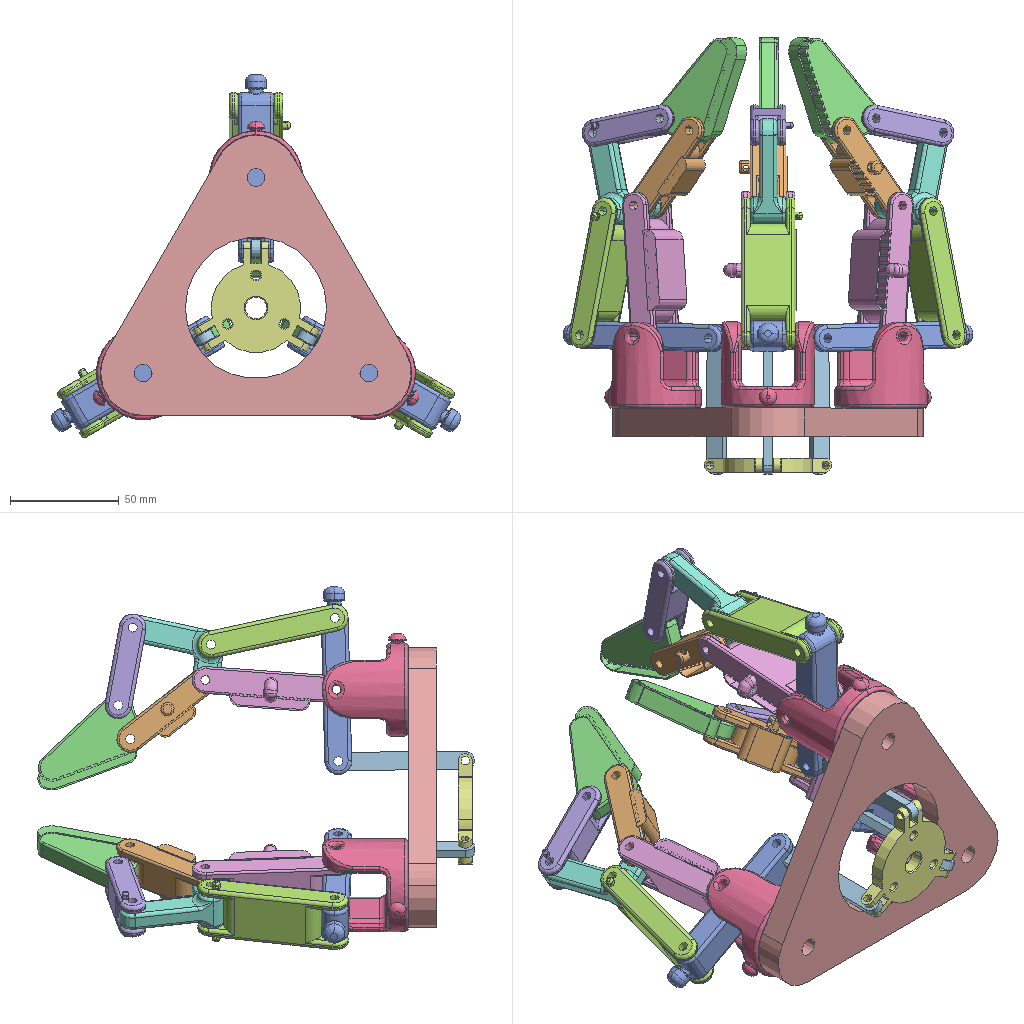Assembly | SolidWorks | 10 different items | 26 placed | box 189 x 201 x 167 mm
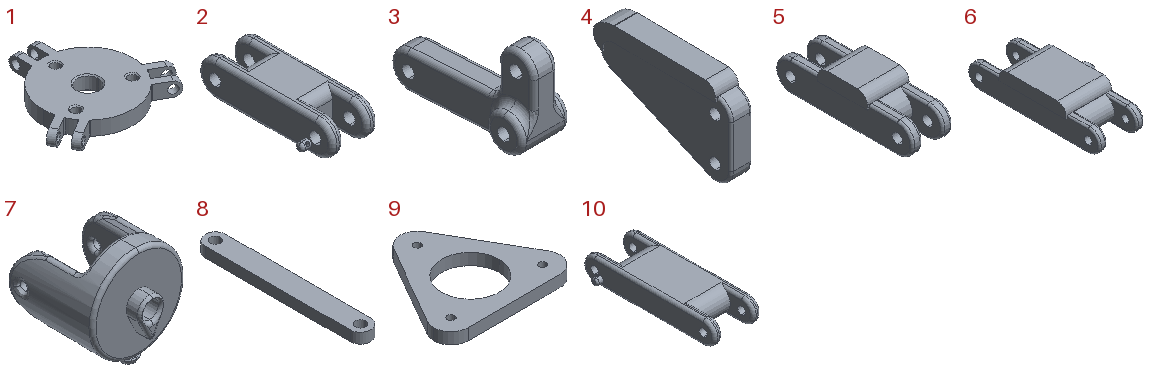Parts list (item | quantity | size | volume | features):
1 | x1 | 58.764 x 51.19 x 6.5 mm | 8922 mm3 | features ICE 5, Chamfer 2, CirPattern 2, Extrusion 1, Fillet 1, Scale 1
2 | x3 | 19.812 x 48.771 x 12.383 mm | 6676 mm3 | features ICE 4, Fillet 3, 3DProfileFeature 2, Extrusion 1, Scale 1
3 | x3 | 16.51 x 49.289 x 30.864 mm | 6856 mm3 | features Fillet 3, ICE 3, 3DProfileFeature 2, Extrusion 1, Scale 1
4 | x3 | 8.915 x 52.717 x 33.373 mm | 8638 mm3 | features ICE 5, CirPattern 1, Extrusion 1, Fillet 1, LPattern 1, Scale 1
5 | x3 | 22.123 x 56.398 x 16.345 mm | 8448 mm3 | features ICE 7, 3DProfileFeature 2, Fillet 2, Extrusion 1, LPattern 1, Scale 1
6 | x3 | 33.423 x 72.908 x 17.17 mm | 16126 mm3 | features ICE 5, 3DProfileFeature 2, Fillet 2, Extrusion 1, LPattern 1, Scale 1, Sweep 1
7 | x3 | 42.926 x 46.228 x 47.219 mm | 24971 mm3 | features Fillet 11, ICE 9, Extrusion 1, Scale 1
8 | x3 | 8.32 x 66.82 x 4.134 mm | 2126 mm3 | features Extrusion 1, Scale 1
9 | x1 | 143 x 129.067 x 13 mm | 109293 mm3 | features Extrusion 1, ICE 1, Scale 1
10 | x3 | 28.067 x 70.63 x 12.383 mm | 15312 mm3 | features ICE 4, 3DProfileFeature 2, Fillet 2, Extrusion 1, Scale 1
Mates (type | each side: item.copy, entity, surface, feature):
Concentric | 10.1 face cylinder Cut-Extrude1 | 3.1 face cylinder Cut-Extrude2
Coincident | 10.1 face plane Cut-Extrude2 | 3.1 face plane Boss-Extrude2
Concentric | 6.1 face cylinder Cut-Extrude1 | 5.1 face cylinder Cut-Extrude1
Concentric | 6.1 face cylinder Cut-Extrude1 | 3.1 face cylinder Cut-Extrude1
Coincident | 6.1 face plane Cut-Extrude2 | 5.1 face plane Boss-Extrude1
Concentric | 6.1 face cylinder Cut-Extrude1 | 7.1 face cylinder Bolt Hole
Coincident | 6.1 face plane Boss-Extrude1 | 7.1 face plane Side Wall
Coincident | 3.1 face plane Boss-Extrude1 | 5.1 face plane Cut-Extrude2
Concentric | 3.1 face cylinder Cut-Extrude1 | 2.1 face cylinder Cut-Extrude1
Concentric | 5.1 face cylinder Cut-Extrude1 | 4.1 face cylinder Cut-Extrude1
Coincident | 5.1 face plane Cut-Extrude2 | 4.1 face plane Boss-Extrude1
Concentric | 2.1 face cylinder Cut-Extrude1 | 4.1 face cylinder Cut-Extrude1
Coincident | 2.1 face plane Cut-Extrude2 | 4.1 face plane Boss-Extrude1
Parallel | 9.1 face plane Boss-Extrude1 | assembly plane
Coincident | 9.1 plane | assembly plane | 2 times
Concentric | 9.1 face cylinder Boss-Extrude1 | 7.1 face cylinder Base plate
Concentric | 9.1 face cylinder Cut-Extrude1 | 7.1 face cylinder Lip
Coincident | 9.1 face plane Cut-Extrude1 | 7.1 face plane Lip
Coincident | 9.1 face plane Boss-Extrude1 | 7.1 face plane Base plate
Parallel | 9.1 face plane Boss-Extrude1 | 1.1 face plane Boss-Extrude1
Concentric | 8.1 face cylinder Boss-Extrude1 | 1.1 face cylinder Cut-Extrude1
Concentric | 9.1 face cylinder Boss-Extrude1 | 1.1 face cylinder Cut-Extrude4